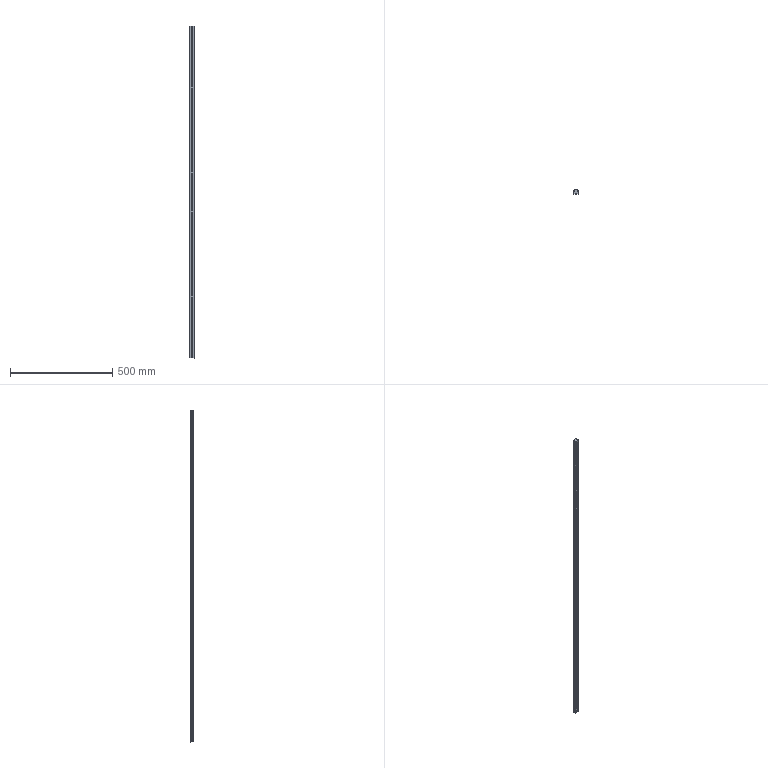Part | SolidWorks | features MoveFace 3, BaseBody 1, HoleWzd 1 | 1 solid | 246 faces | box 23 x 18 x 1620 mm | volume 561456 mm3 | plane 130 | cylinder 116 | commonest cylinder face diameters 11 x54 6.6 x48 7 x6 1 x4 4 x4